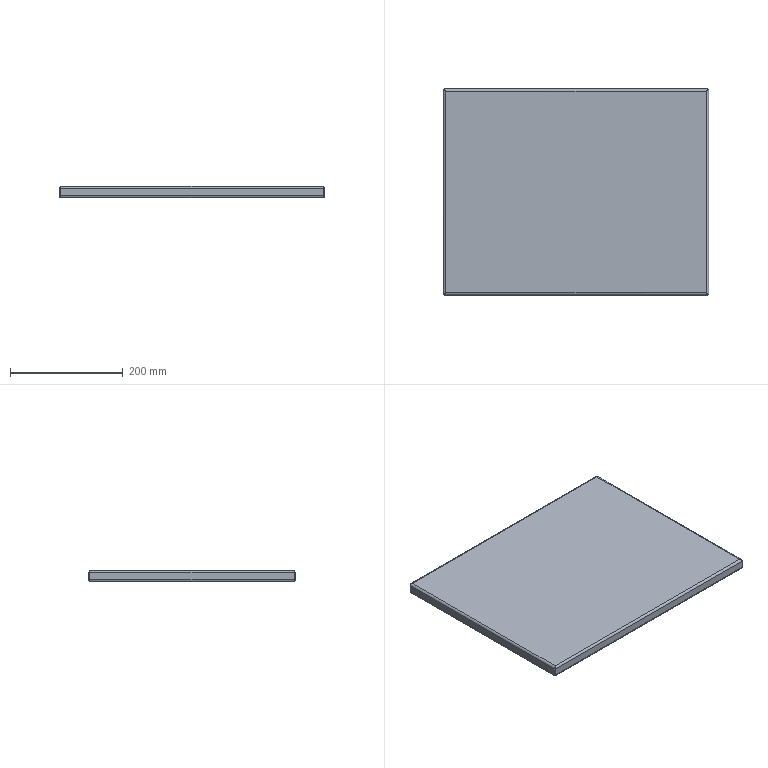Part | STEP file | 750078421 | 1 solid | 62 faces | box 471 x 366 x 20 mm | volume 448317 mm3 | plane 46 | cylinder 16 | commonest cylinder face diameters 2 x4 4 x4 6 x4 8 x4